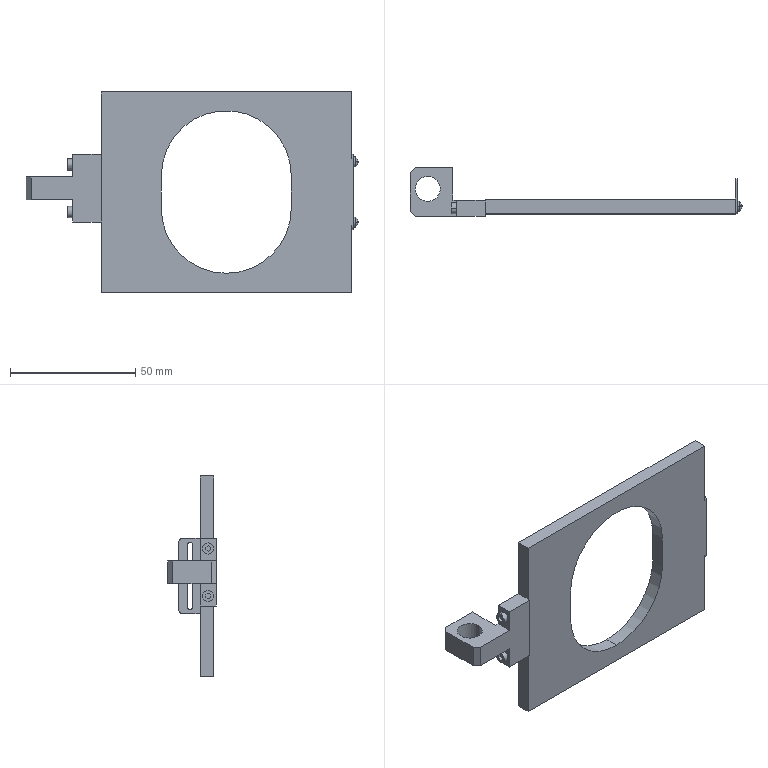Part | SolidWorks | features ICE 10, Revolution 2, Extrusion 1 | 1 solid | 92 faces | box 132.782 x 19.5 x 80 mm | volume 33329 mm3 | plane 64 | cylinder 20 | torus 8 | commonest cylinder face diameters 3 x4 4 x4 4.5 x4 2 x3 52 x3 10 x2